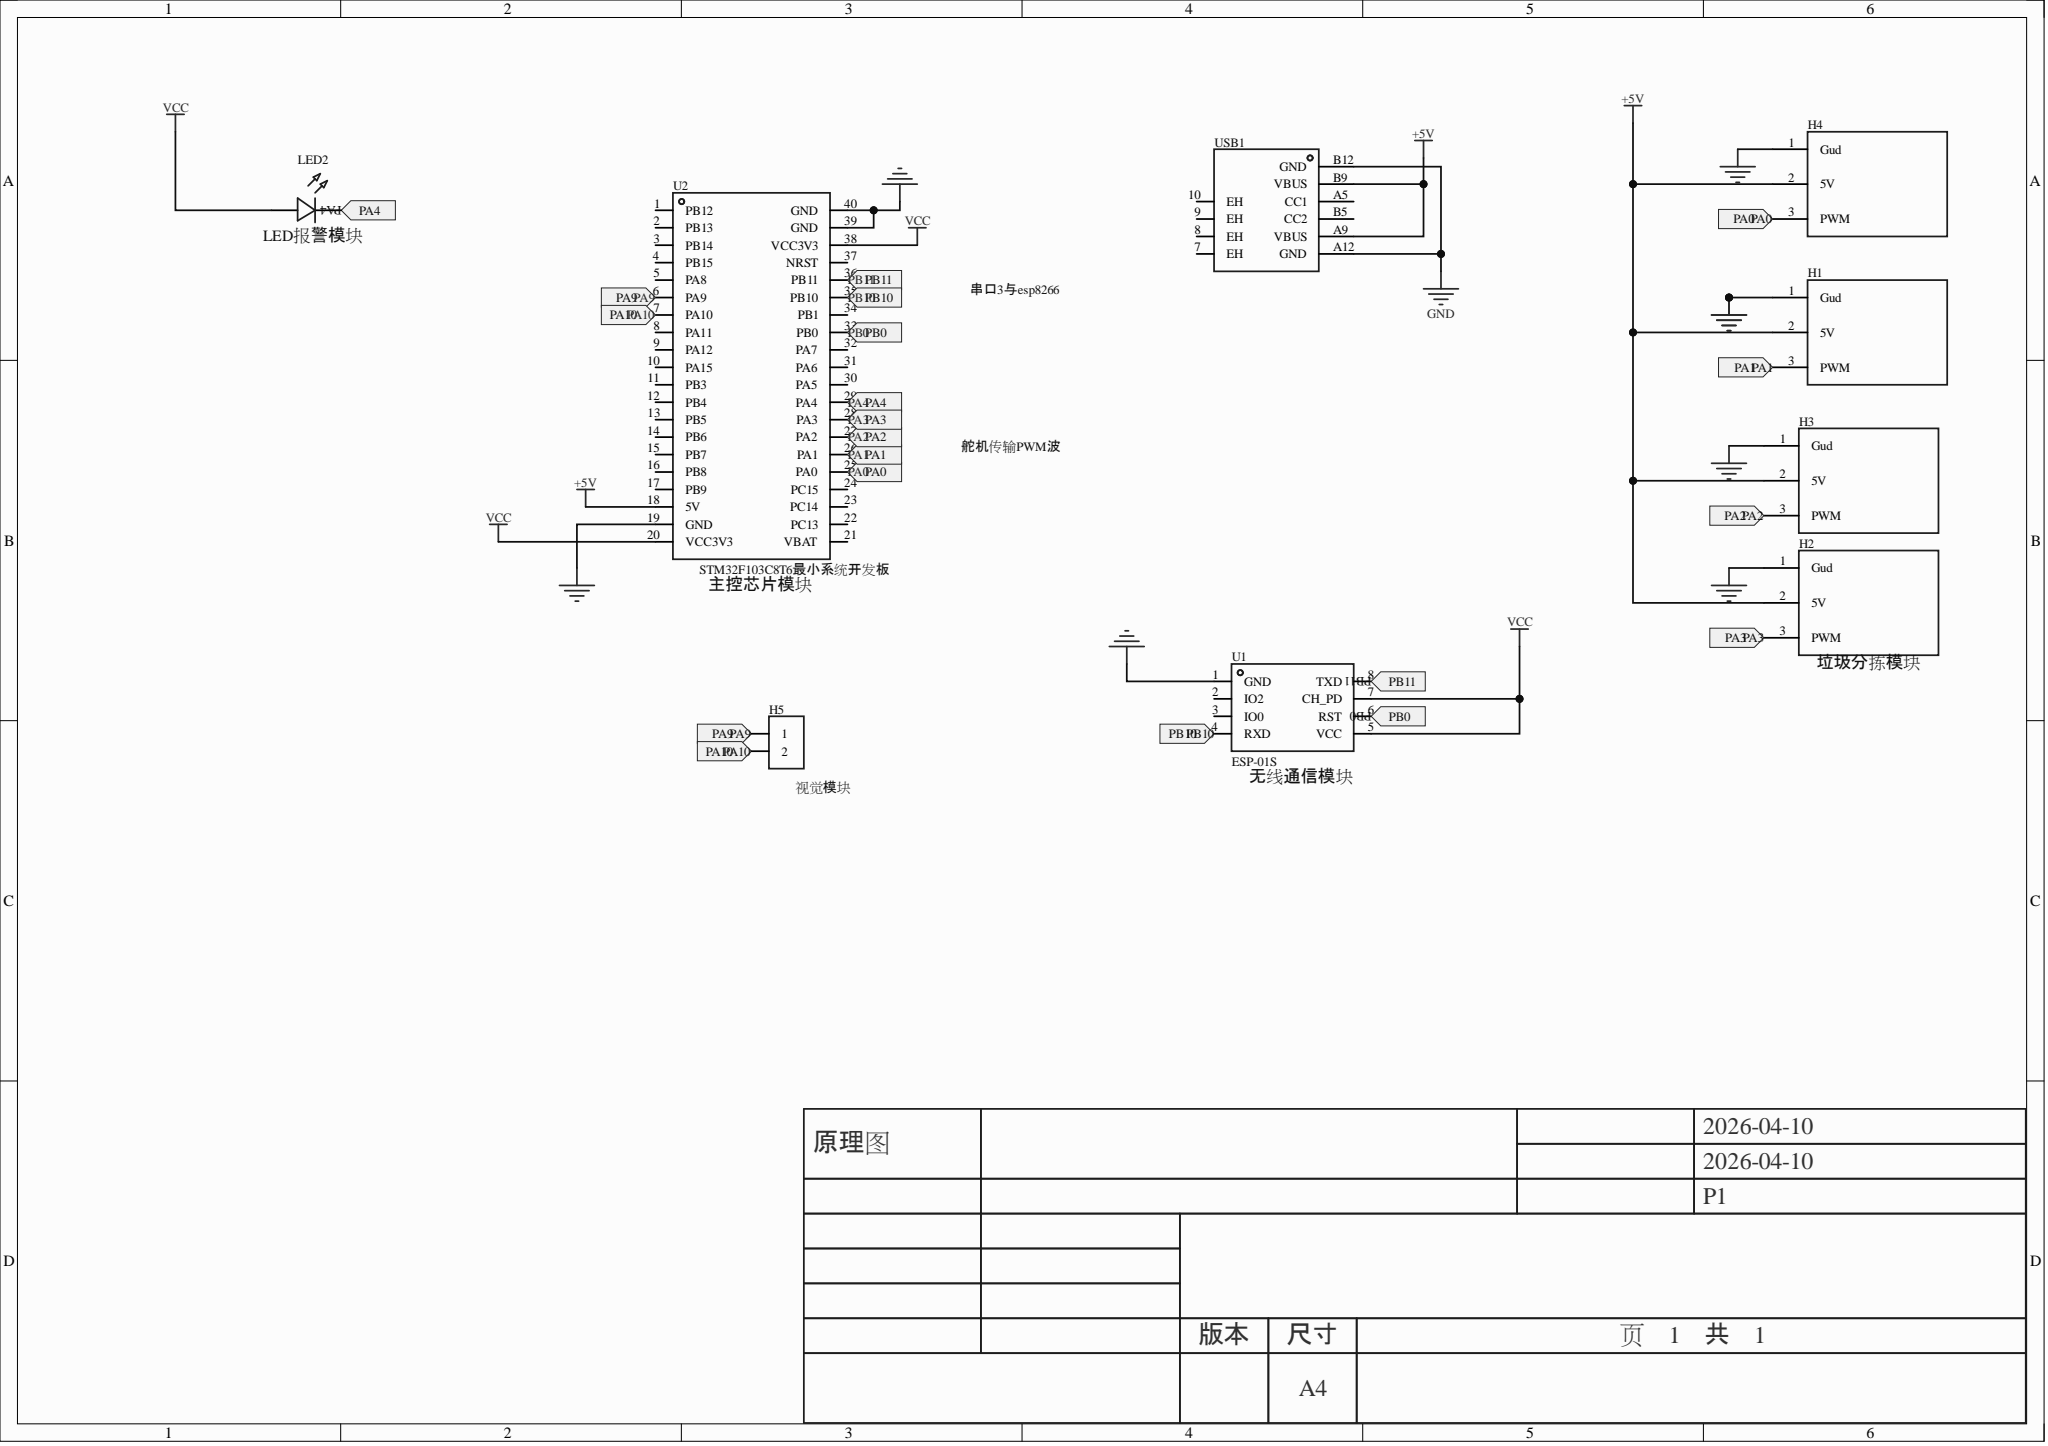Circuit board | Altium Designer | 9 parts | 13 nets
Bill of materials:
Comment,Description,Designator,Footprint,LibRef,Quantity
"","","H1, H2, H3, H4","HDR-TH_3P-P2.54-V-F","GS90","4"
"","","H5","HDR-TH_2P-P2.54-V-F","HDR-F_2.54_1x2P","1"
"","","LED2","LED_TH-3mm","LED_TH-R_3mm","1"
"ESP-01S","","U1","WIFIM-TH_ESP-01S","ESP-01S_C111009","1"
"STM32F103C8T6最小系统开发板","","U2","CONN-TH_L53.3-W22.9_STM32F103C8T6-CARD","STM32F103C8T6-Card","1"
"","","USB1","USB_ TYPE-C-6P","USB_ Type-C-6P","1"
Netlist (Protel format):
[
H1
HDR-TH_3P-P2.54-V-F




]
[
H2
HDR-TH_3P-P2.54-V-F




]
[
H3
HDR-TH_3P-P2.54-V-F




]
[
H4
HDR-TH_3P-P2.54-V-F




]
[
H5
HDR-TH_2P-P2.54-V-F




]
[
LED2
LED_TH-3mm




]
[
U1
WIFIM-TH_ESP-01S
ESP-01S



]
[
U2
CONN-TH_L53.3-W22.9_STM32F103C8T6-CARD
STM32F103C8T6最小系统开发板



]
[
USB1
USB_ TYPE-C-6P




]
(
VCC
LED2-1
U1-5
U1-7
U2-20
U2-38
)
(
PB11
U1-8
U2-36
)
(
PB10
U1-4
U2-35
)
(
PB0
U1-6
U2-33
)
(
PA10
H5-2
U2-7
)
(
PA9
H5-1
U2-6
)
(
PA4
LED2-2
U2-29
)
(
PA3
H2-3
U2-28
)
(
PA2
H3-3
U2-27
)
(
PA1
H1-3
U2-26
)
(
PA0
H4-3
U2-25
)
(
GND
H1-1
H2-1
H3-1
H4-1
U1-1
U2-19
U2-39
U2-40
USB1-A12
USB1-B12
)
(
+5V
H1-2
H2-2
H3-2
H4-2
U2-18
USB1-A9
USB1-B9
)